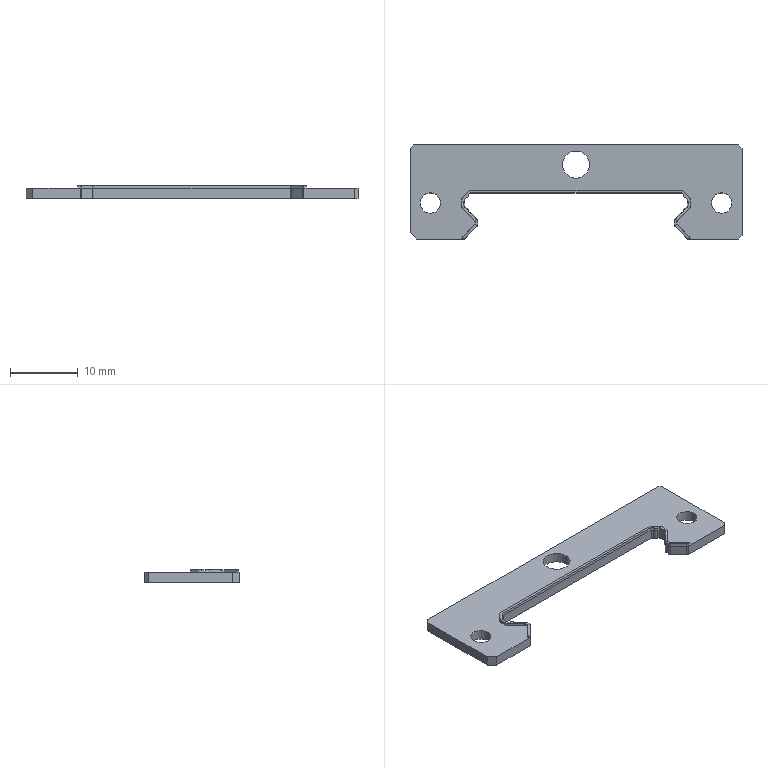Part | SolidWorks | features BaseBody 1 | 1 solid | 104 faces | box 49 x 13.9 x 1.9 mm | volume 669.642 mm3 | plane 57 | cone 25 | cylinder 22 | commonest cylinder face diameters 1 x10 0.77 x6 3 x4 4 x2